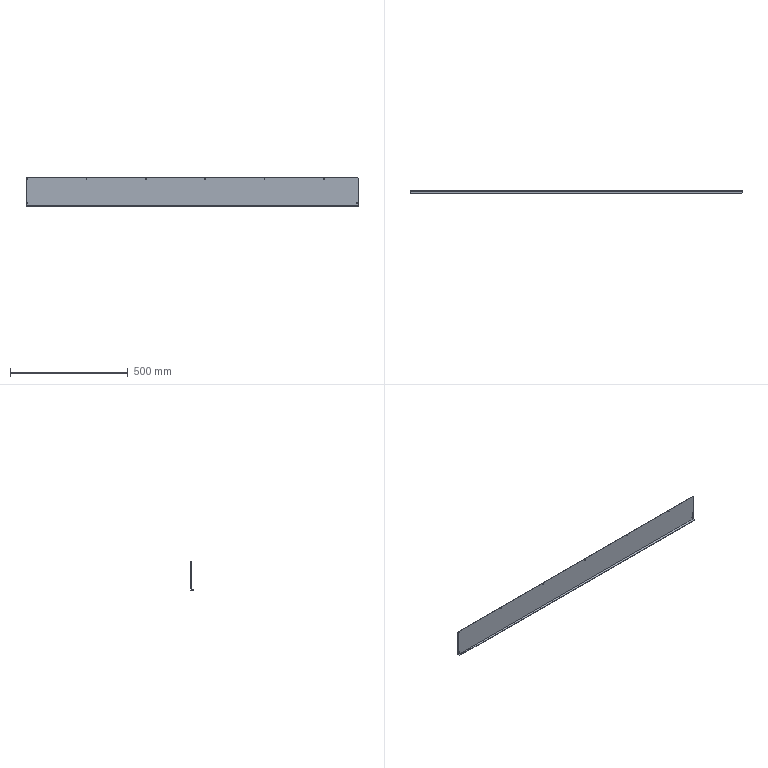Part | NX | 1 solid | 20 faces | box 1410 x 10.5 x 119 mm | volume 359389 mm3 | plane 12 | cylinder 8 | commonest cylinder face diameters 3.4 x8
STEP:
#1=CARTESIAN_POINT('',(-705.,0.,-117.));
#2=VERTEX_POINT('',#1);
#3=CARTESIAN_POINT('',(-705.,-6.5,-117.));
#4=VERTEX_POINT('',#3);
#5=CARTESIAN_POINT('',(-705.,0.,-117.));
#6=DIRECTION('',(0.,-1.,0.));
#7=VECTOR('',#6,1000.);
#8=LINE('',#5,#7);
#9=EDGE_CURVE('',#2,#4,#8,.T.);
#10=ORIENTED_EDGE('',*,*,#9,.T.);
#11=CARTESIAN_POINT('',(-703.,-8.5,-117.));
#12=VERTEX_POINT('',#11);
#13=CARTESIAN_POINT('',(-705.,-6.5,-117.));
#14=DIRECTION('',(-0.7071,0.7071,0.));
#15=VECTOR('',#14,1000.);
#16=LINE('',#13,#15);
#17=EDGE_CURVE('',#4,#12,#16,.F.);
#18=ORIENTED_EDGE('',*,*,#17,.T.);
#19=CARTESIAN_POINT('',(703.,-8.5,-117.));
#20=VERTEX_POINT('',#19);
#21=CARTESIAN_POINT('',(705.,-8.5,-117.));
#22=DIRECTION('',(-1.,0.,0.));
#23=VECTOR('',#22,1000.);
#24=LINE('',#21,#23);
#25=EDGE_CURVE('',#20,#12,#24,.T.);
#26=ORIENTED_EDGE('',*,*,#25,.F.);
#27=CARTESIAN_POINT('',(705.,-6.5,-117.));
#28=VERTEX_POINT('',#27);
#29=CARTESIAN_POINT('',(703.,-8.5,-117.));
#30=DIRECTION('',(0.7071,0.7071,0.));
#31=VECTOR('',#30,1000.);
#32=LINE('',#29,#31);
#33=EDGE_CURVE('',#20,#28,#32,.T.);
#34=ORIENTED_EDGE('',*,*,#33,.T.);
#35=CARTESIAN_POINT('',(705.,0.,-117.));
#36=VERTEX_POINT('',#35);
#37=CARTESIAN_POINT('',(705.,0.,-117.));
#38=DIRECTION('',(0.,-1.,0.));
#39=VECTOR('',#38,1000.);
#40=LINE('',#37,#39);
#41=EDGE_CURVE('',#36,#28,#40,.T.);
#42=ORIENTED_EDGE('',*,*,#41,.F.);
#43=CARTESIAN_POINT('',(705.,0.,-117.));
#44=DIRECTION('',(-1.,0.,0.));
#45=VECTOR('',#44,1000.);
#46=LINE('',#43,#45);
#47=EDGE_CURVE('',#36,#2,#46,.T.);
#48=ORIENTED_EDGE('',*,*,#47,.T.);
#49=EDGE_LOOP('',(#10,#18,#26,#34,#42,#48));
#50=FACE_BOUND('',#49,.T.);
#51=CARTESIAN_POINT('',(705.,0.,-117.));
#52=DIRECTION('',(0.,0.,-1.));
#53=DIRECTION('',(-1.,0.,0.));
#54=AXIS2_PLACEMENT_3D('',#51,#52,#53);
#55=PLANE('',#54);
#56=ADVANCED_FACE('',(#50),#55,.F.);
#57=ORIENTED_EDGE('',*,*,#25,.T.);
#58=CARTESIAN_POINT('',(-703.,-8.5,-119.));
#59=VERTEX_POINT('',#58);
#60=CARTESIAN_POINT('',(-703.,-8.5,-119.));
#61=DIRECTION('',(0.,0.,-1.));
#62=VECTOR('',#61,1000.);
#63=LINE('',#60,#62);
#64=EDGE_CURVE('',#12,#59,#63,.T.);
#65=ORIENTED_EDGE('',*,*,#64,.T.);
#66=CARTESIAN_POINT('',(703.,-8.5,-119.));
#67=VERTEX_POINT('',#66);
#68=CARTESIAN_POINT('',(705.,-8.5,-119.));
#69=DIRECTION('',(-1.,0.,0.));
#70=VECTOR('',#69,1000.);
#71=LINE('',#68,#70);
#72=EDGE_CURVE('',#67,#59,#71,.T.);
#73=ORIENTED_EDGE('',*,*,#72,.F.);
#74=CARTESIAN_POINT('',(703.,-8.5,-117.));
#75=DIRECTION('',(0.,0.,1.));
#76=VECTOR('',#75,1000.);
#77=LINE('',#74,#76);
#78=EDGE_CURVE('',#67,#20,#77,.T.);
#79=ORIENTED_EDGE('',*,*,#78,.T.);
#80=EDGE_LOOP('',(#57,#65,#73,#79));
#81=FACE_BOUND('',#80,.T.);
#82=CARTESIAN_POINT('',(705.,-8.5,-119.));
#83=DIRECTION('',(0.,-1.,0.));
#84=DIRECTION('',(0.,0.,-1.));
#85=AXIS2_PLACEMENT_3D('',#82,#83,#84);
#86=PLANE('',#85);
#87=ADVANCED_FACE('',(#81),#86,.T.);
#88=ORIENTED_EDGE('',*,*,#72,.T.);
#89=CARTESIAN_POINT('',(-705.,-6.5,-119.));
#90=VERTEX_POINT('',#89);
#91=CARTESIAN_POINT('',(-3.25,-708.25,-119.));
#92=DIRECTION('',(0.7071,-0.7071,0.));
#93=VECTOR('',#92,1000.);
#94=LINE('',#91,#93);
#95=EDGE_CURVE('',#59,#90,#94,.F.);
#96=ORIENTED_EDGE('',*,*,#95,.T.);
#97=CARTESIAN_POINT('',(-705.,2.,-119.));
#98=VERTEX_POINT('',#97);
#99=CARTESIAN_POINT('',(-705.,0.,-119.));
#100=DIRECTION('',(0.,1.,0.));
#101=VECTOR('',#100,1000.);
#102=LINE('',#99,#101);
#103=EDGE_CURVE('',#98,#90,#102,.F.);
#104=ORIENTED_EDGE('',*,*,#103,.F.);
#105=CARTESIAN_POINT('',(705.,2.,-119.));
#106=VERTEX_POINT('',#105);
#107=CARTESIAN_POINT('',(705.,2.,-119.));
#108=DIRECTION('',(-1.,0.,0.));
#109=VECTOR('',#108,1000.);
#110=LINE('',#107,#109);
#111=EDGE_CURVE('',#106,#98,#110,.T.);
#112=ORIENTED_EDGE('',*,*,#111,.F.);
#113=CARTESIAN_POINT('',(705.,-6.5,-119.));
#114=VERTEX_POINT('',#113);
#115=CARTESIAN_POINT('',(705.,0.,-119.));
#116=DIRECTION('',(0.,1.,0.));
#117=VECTOR('',#116,1000.);
#118=LINE('',#115,#117);
#119=EDGE_CURVE('',#106,#114,#118,.F.);
#120=ORIENTED_EDGE('',*,*,#119,.T.);
#121=CARTESIAN_POINT('',(708.25,-3.25,-119.));
#122=DIRECTION('',(-0.7071,-0.7071,0.));
#123=VECTOR('',#122,1000.);
#124=LINE('',#121,#123);
#125=EDGE_CURVE('',#114,#67,#124,.T.);
#126=ORIENTED_EDGE('',*,*,#125,.T.);
#127=EDGE_LOOP('',(#88,#96,#104,#112,#120,#126));
#128=FACE_BOUND('',#127,.T.);
#129=CARTESIAN_POINT('',(705.,0.,-119.));
#130=DIRECTION('',(0.,0.,-1.));
#131=DIRECTION('',(-1.,0.,0.));
#132=AXIS2_PLACEMENT_3D('',#129,#130,#131);
#133=PLANE('',#132);
#134=ADVANCED_FACE('',(#128),#133,.T.);
#135=CARTESIAN_POINT('',(-700.,2.,-103.3));
#136=VERTEX_POINT('',#135);
#137=CARTESIAN_POINT('',(-700.,2.,-105.));
#138=DIRECTION('',(0.,1.,0.));
#139=DIRECTION('',(0.,0.,1.));
#140=AXIS2_PLACEMENT_3D('',#137,#138,#139);
#141=CIRCLE('',#140,1.7);
#142=EDGE_CURVE('',#136,#136,#141,.T.);
#143=ORIENTED_EDGE('',*,*,#142,.F.);
#144=EDGE_LOOP('',(#143));
#145=FACE_BOUND('',#144,.T.);
#146=CARTESIAN_POINT('',(700.,2.,-103.3));
#147=VERTEX_POINT('',#146);
#148=CARTESIAN_POINT('',(700.,2.,-105.));
#149=DIRECTION('',(0.,1.,0.));
#150=DIRECTION('',(0.,0.,1.));
#151=AXIS2_PLACEMENT_3D('',#148,#149,#150);
#152=CIRCLE('',#151,1.7);
#153=EDGE_CURVE('',#147,#147,#152,.T.);
#154=ORIENTED_EDGE('',*,*,#153,.F.);
#155=EDGE_LOOP('',(#154));
#156=FACE_BOUND('',#155,.T.);
#157=CARTESIAN_POINT('',(-448.,2.,-3.3));
#158=VERTEX_POINT('',#157);
#159=CARTESIAN_POINT('',(-448.,2.,-5.));
#160=DIRECTION('',(0.,1.,0.));
#161=DIRECTION('',(0.,0.,1.));
#162=AXIS2_PLACEMENT_3D('',#159,#160,#161);
#163=CIRCLE('',#162,1.7);
#164=EDGE_CURVE('',#158,#158,#163,.T.);
#165=ORIENTED_EDGE('',*,*,#164,.F.);
#166=EDGE_LOOP('',(#165));
#167=FACE_BOUND('',#166,.T.);
#168=CARTESIAN_POINT('',(-700.,2.,-3.3));
#169=VERTEX_POINT('',#168);
#170=CARTESIAN_POINT('',(-700.,2.,-5.));
#171=DIRECTION('',(0.,1.,0.));
#172=DIRECTION('',(0.,0.,1.));
#173=AXIS2_PLACEMENT_3D('',#170,#171,#172);
#174=CIRCLE('',#173,1.7);
#175=EDGE_CURVE('',#169,#169,#174,.T.);
#176=ORIENTED_EDGE('',*,*,#175,.F.);
#177=EDGE_LOOP('',(#176));
#178=FACE_BOUND('',#177,.T.);
#179=CARTESIAN_POINT('',(703.,2.,0.));
#180=VERTEX_POINT('',#179);
#181=CARTESIAN_POINT('',(-703.,2.,0.));
#182=VERTEX_POINT('',#181);
#183=CARTESIAN_POINT('',(705.,2.,0.));
#184=DIRECTION('',(-1.,0.,0.));
#185=VECTOR('',#184,1000.);
#186=LINE('',#183,#185);
#187=EDGE_CURVE('',#180,#182,#186,.T.);
#188=ORIENTED_EDGE('',*,*,#187,.F.);
#189=CARTESIAN_POINT('',(705.,2.,-2.));
#190=VERTEX_POINT('',#189);
#191=CARTESIAN_POINT('',(704.,2.,-1.));
#192=DIRECTION('',(0.7071,0.,-0.7071));
#193=VECTOR('',#192,1000.);
#194=LINE('',#191,#193);
#195=EDGE_CURVE('',#180,#190,#194,.T.);
#196=ORIENTED_EDGE('',*,*,#195,.T.);
#197=CARTESIAN_POINT('',(705.,2.,0.));
#198=DIRECTION('',(0.,0.,-1.));
#199=VECTOR('',#198,1000.);
#200=LINE('',#197,#199);
#201=EDGE_CURVE('',#190,#106,#200,.T.);
#202=ORIENTED_EDGE('',*,*,#201,.T.);
#203=ORIENTED_EDGE('',*,*,#111,.T.);
#204=CARTESIAN_POINT('',(-705.,2.,-2.));
#205=VERTEX_POINT('',#204);
#206=CARTESIAN_POINT('',(-705.,2.,0.));
#207=DIRECTION('',(0.,0.,-1.));
#208=VECTOR('',#207,1000.);
#209=LINE('',#206,#208);
#210=EDGE_CURVE('',#205,#98,#209,.T.);
#211=ORIENTED_EDGE('',*,*,#210,.F.);
#212=CARTESIAN_POINT('',(1.,2.,704.));
#213=DIRECTION('',(-0.7071,0.,-0.7071));
#214=VECTOR('',#213,1000.);
#215=LINE('',#212,#214);
#216=EDGE_CURVE('',#205,#182,#215,.F.);
#217=ORIENTED_EDGE('',*,*,#216,.T.);
#218=EDGE_LOOP('',(#188,#196,#202,#203,#211,#217));
#219=FACE_BOUND('',#218,.T.);
#220=CARTESIAN_POINT('',(-196.,2.,-3.3));
#221=VERTEX_POINT('',#220);
#222=CARTESIAN_POINT('',(-196.,2.,-5.));
#223=DIRECTION('',(0.,1.,0.));
#224=DIRECTION('',(0.,0.,1.));
#225=AXIS2_PLACEMENT_3D('',#222,#223,#224);
#226=CIRCLE('',#225,1.7);
#227=EDGE_CURVE('',#221,#221,#226,.T.);
#228=ORIENTED_EDGE('',*,*,#227,.F.);
#229=EDGE_LOOP('',(#228));
#230=FACE_BOUND('',#229,.T.);
#231=CARTESIAN_POINT('',(56.,2.,-3.3));
#232=VERTEX_POINT('',#231);
#233=CARTESIAN_POINT('',(56.,2.,-5.));
#234=DIRECTION('',(0.,1.,0.));
#235=DIRECTION('',(0.,0.,1.));
#236=AXIS2_PLACEMENT_3D('',#233,#234,#235);
#237=CIRCLE('',#236,1.7);
#238=EDGE_CURVE('',#232,#232,#237,.T.);
#239=ORIENTED_EDGE('',*,*,#238,.F.);
#240=EDGE_LOOP('',(#239));
#241=FACE_BOUND('',#240,.T.);
#242=CARTESIAN_POINT('',(308.,2.,-3.3));
#243=VERTEX_POINT('',#242);
#244=CARTESIAN_POINT('',(308.,2.,-5.));
#245=DIRECTION('',(0.,1.,0.));
#246=DIRECTION('',(0.,0.,1.));
#247=AXIS2_PLACEMENT_3D('',#244,#245,#246);
#248=CIRCLE('',#247,1.7);
#249=EDGE_CURVE('',#243,#243,#248,.T.);
#250=ORIENTED_EDGE('',*,*,#249,.F.);
#251=EDGE_LOOP('',(#250));
#252=FACE_BOUND('',#251,.T.);
#253=CARTESIAN_POINT('',(560.,2.,-3.3));
#254=VERTEX_POINT('',#253);
#255=CARTESIAN_POINT('',(560.,2.,-5.));
#256=DIRECTION('',(0.,1.,0.));
#257=DIRECTION('',(0.,0.,1.));
#258=AXIS2_PLACEMENT_3D('',#255,#256,#257);
#259=CIRCLE('',#258,1.7);
#260=EDGE_CURVE('',#254,#254,#259,.T.);
#261=ORIENTED_EDGE('',*,*,#260,.F.);
#262=EDGE_LOOP('',(#261));
#263=FACE_BOUND('',#262,.T.);
#264=CARTESIAN_POINT('',(705.,2.,0.));
#265=DIRECTION('',(0.,1.,0.));
#266=DIRECTION('',(0.,0.,1.));
#267=AXIS2_PLACEMENT_3D('',#264,#265,#266);
#268=PLANE('',#267);
#269=ADVANCED_FACE('',(#145,#156,#167,#178,#219,#230,#241,#252,#263),#268,.T.);
#270=CARTESIAN_POINT('',(703.,0.,0.));
#271=VERTEX_POINT('',#270);
#272=CARTESIAN_POINT('',(-703.,0.,0.));
#273=VERTEX_POINT('',#272);
#274=CARTESIAN_POINT('',(705.,0.,0.));
#275=DIRECTION('',(-1.,0.,0.));
#276=VECTOR('',#275,1000.);
#277=LINE('',#274,#276);
#278=EDGE_CURVE('',#271,#273,#277,.T.);
#279=ORIENTED_EDGE('',*,*,#278,.F.);
#280=CARTESIAN_POINT('',(703.,2.,0.));
#281=DIRECTION('',(0.,1.,0.));
#282=VECTOR('',#281,1000.);
#283=LINE('',#280,#282);
#284=EDGE_CURVE('',#271,#180,#283,.T.);
#285=ORIENTED_EDGE('',*,*,#284,.T.);
#286=ORIENTED_EDGE('',*,*,#187,.T.);
#287=CARTESIAN_POINT('',(-703.,0.,0.));
#288=DIRECTION('',(0.,-1.,0.));
#289=VECTOR('',#288,1000.);
#290=LINE('',#287,#289);
#291=EDGE_CURVE('',#182,#273,#290,.T.);
#292=ORIENTED_EDGE('',*,*,#291,.T.);
#293=EDGE_LOOP('',(#279,#285,#286,#292));
#294=FACE_BOUND('',#293,.T.);
#295=CARTESIAN_POINT('',(705.,0.,0.));
#296=DIRECTION('',(0.,0.,1.));
#297=DIRECTION('',(1.,0.,0.));
#298=AXIS2_PLACEMENT_3D('',#295,#296,#297);
#299=PLANE('',#298);
#300=ADVANCED_FACE('',(#294),#299,.T.);
#301=CARTESIAN_POINT('',(-700.,0.,-103.3));
#302=VERTEX_POINT('',#301);
#303=CARTESIAN_POINT('',(-700.,0.,-105.));
#304=DIRECTION('',(0.,1.,0.));
#305=DIRECTION('',(0.,0.,1.));
#306=AXIS2_PLACEMENT_3D('',#303,#304,#305);
#307=CIRCLE('',#306,1.7);
#308=EDGE_CURVE('',#302,#302,#307,.T.);
#309=ORIENTED_EDGE('',*,*,#308,.T.);
#310=EDGE_LOOP('',(#309));
#311=FACE_BOUND('',#310,.T.);
#312=CARTESIAN_POINT('',(700.,0.,-103.3));
#313=VERTEX_POINT('',#312);
#314=CARTESIAN_POINT('',(700.,0.,-105.));
#315=DIRECTION('',(0.,1.,0.));
#316=DIRECTION('',(0.,0.,1.));
#317=AXIS2_PLACEMENT_3D('',#314,#315,#316);
#318=CIRCLE('',#317,1.7);
#319=EDGE_CURVE('',#313,#313,#318,.T.);
#320=ORIENTED_EDGE('',*,*,#319,.T.);
#321=EDGE_LOOP('',(#320));
#322=FACE_BOUND('',#321,.T.);
#323=CARTESIAN_POINT('',(-448.,0.,-3.3));
#324=VERTEX_POINT('',#323);
#325=CARTESIAN_POINT('',(-448.,0.,-5.));
#326=DIRECTION('',(0.,1.,0.));
#327=DIRECTION('',(0.,0.,1.));
#328=AXIS2_PLACEMENT_3D('',#325,#326,#327);
#329=CIRCLE('',#328,1.7);
#330=EDGE_CURVE('',#324,#324,#329,.T.);
#331=ORIENTED_EDGE('',*,*,#330,.T.);
#332=EDGE_LOOP('',(#331));
#333=FACE_BOUND('',#332,.T.);
#334=CARTESIAN_POINT('',(-700.,0.,-3.3));
#335=VERTEX_POINT('',#334);
#336=CARTESIAN_POINT('',(-700.,0.,-5.));
#337=DIRECTION('',(0.,1.,0.));
#338=DIRECTION('',(0.,0.,1.));
#339=AXIS2_PLACEMENT_3D('',#336,#337,#338);
#340=CIRCLE('',#339,1.7);
#341=EDGE_CURVE('',#335,#335,#340,.T.);
#342=ORIENTED_EDGE('',*,*,#341,.T.);
#343=EDGE_LOOP('',(#342));
#344=FACE_BOUND('',#343,.T.);
#345=CARTESIAN_POINT('',(705.,0.,-2.));
#346=VERTEX_POINT('',#345);
#347=CARTESIAN_POINT('',(705.,0.,0.));
#348=DIRECTION('',(0.,0.,-1.));
#349=VECTOR('',#348,1000.);
#350=LINE('',#347,#349);
#351=EDGE_CURVE('',#346,#36,#350,.T.);
#352=ORIENTED_EDGE('',*,*,#351,.F.);
#353=CARTESIAN_POINT('',(703.,0.,0.));
#354=DIRECTION('',(-0.7071,0.,0.7071));
#355=VECTOR('',#354,1000.);
#356=LINE('',#353,#355);
#357=EDGE_CURVE('',#346,#271,#356,.T.);
#358=ORIENTED_EDGE('',*,*,#357,.T.);
#359=ORIENTED_EDGE('',*,*,#278,.T.);
#360=CARTESIAN_POINT('',(-705.,0.,-2.));
#361=VERTEX_POINT('',#360);
#362=CARTESIAN_POINT('',(-705.,0.,-2.));
#363=DIRECTION('',(0.7071,0.,0.7071));
#364=VECTOR('',#363,1000.);
#365=LINE('',#362,#364);
#366=EDGE_CURVE('',#273,#361,#365,.F.);
#367=ORIENTED_EDGE('',*,*,#366,.T.);
#368=CARTESIAN_POINT('',(-705.,0.,0.));
#369=DIRECTION('',(0.,0.,-1.));
#370=VECTOR('',#369,1000.);
#371=LINE('',#368,#370);
#372=EDGE_CURVE('',#361,#2,#371,.T.);
#373=ORIENTED_EDGE('',*,*,#372,.T.);
#374=ORIENTED_EDGE('',*,*,#47,.F.);
#375=EDGE_LOOP('',(#352,#358,#359,#367,#373,#374));
#376=FACE_BOUND('',#375,.T.);
#377=CARTESIAN_POINT('',(-196.,0.,-3.3));
#378=VERTEX_POINT('',#377);
#379=CARTESIAN_POINT('',(-196.,0.,-5.));
#380=DIRECTION('',(0.,1.,0.));
#381=DIRECTION('',(0.,0.,1.));
#382=AXIS2_PLACEMENT_3D('',#379,#380,#381);
#383=CIRCLE('',#382,1.7);
#384=EDGE_CURVE('',#378,#378,#383,.T.);
#385=ORIENTED_EDGE('',*,*,#384,.T.);
#386=EDGE_LOOP('',(#385));
#387=FACE_BOUND('',#386,.T.);
#388=CARTESIAN_POINT('',(56.,0.,-3.3));
#389=VERTEX_POINT('',#388);
#390=CARTESIAN_POINT('',(56.,0.,-5.));
#391=DIRECTION('',(0.,1.,0.));
#392=DIRECTION('',(0.,0.,1.));
#393=AXIS2_PLACEMENT_3D('',#390,#391,#392);
#394=CIRCLE('',#393,1.7);
#395=EDGE_CURVE('',#389,#389,#394,.T.);
#396=ORIENTED_EDGE('',*,*,#395,.T.);
#397=EDGE_LOOP('',(#396));
#398=FACE_BOUND('',#397,.T.);
#399=CARTESIAN_POINT('',(308.,0.,-3.3));
#400=VERTEX_POINT('',#399);
#401=CARTESIAN_POINT('',(308.,0.,-5.));
#402=DIRECTION('',(0.,1.,0.));
#403=DIRECTION('',(0.,0.,1.));
#404=AXIS2_PLACEMENT_3D('',#401,#402,#403);
#405=CIRCLE('',#404,1.7);
#406=EDGE_CURVE('',#400,#400,#405,.T.);
#407=ORIENTED_EDGE('',*,*,#406,.T.);
#408=EDGE_LOOP('',(#407));
#409=FACE_BOUND('',#408,.T.);
#410=CARTESIAN_POINT('',(560.,0.,-3.3));
#411=VERTEX_POINT('',#410);
#412=CARTESIAN_POINT('',(560.,0.,-5.));
#413=DIRECTION('',(0.,1.,0.));
#414=DIRECTION('',(0.,0.,1.));
#415=AXIS2_PLACEMENT_3D('',#412,#413,#414);
#416=CIRCLE('',#415,1.7);
#417=EDGE_CURVE('',#411,#411,#416,.T.);
#418=ORIENTED_EDGE('',*,*,#417,.T.);
#419=EDGE_LOOP('',(#418));
#420=FACE_BOUND('',#419,.T.);
#421=CARTESIAN_POINT('',(705.,0.,0.));
#422=DIRECTION('',(0.,1.,0.));
#423=DIRECTION('',(0.,0.,1.));
#424=AXIS2_PLACEMENT_3D('',#421,#422,#423);
#425=PLANE('',#424);
#426=ADVANCED_FACE('',(#311,#322,#333,#344,#376,#387,#398,#409,#420),#425,.F.);
#427=ORIENTED_EDGE('',*,*,#201,.F.);
#428=CARTESIAN_POINT('',(705.,0.,-2.));
#429=DIRECTION('',(0.,-1.,0.));
#430=VECTOR('',#429,1000.);
#431=LINE('',#428,#430);
#432=EDGE_CURVE('',#190,#346,#431,.T.);
#433=ORIENTED_EDGE('',*,*,#432,.T.);
#434=ORIENTED_EDGE('',*,*,#351,.T.);
#435=ORIENTED_EDGE('',*,*,#41,.T.);
#436=CARTESIAN_POINT('',(705.,-6.5,-119.));
#437=DIRECTION('',(0.,0.,-1.));
#438=VECTOR('',#437,1000.);
#439=LINE('',#436,#438);
#440=EDGE_CURVE('',#28,#114,#439,.T.);
#441=ORIENTED_EDGE('',*,*,#440,.T.);
#442=ORIENTED_EDGE('',*,*,#119,.F.);
#443=EDGE_LOOP('',(#427,#433,#434,#435,#441,#442));
#444=FACE_BOUND('',#443,.T.);
#445=CARTESIAN_POINT('',(705.,0.,0.));
#446=DIRECTION('',(-1.,0.,0.));
#447=DIRECTION('',(0.,0.,1.));
#448=AXIS2_PLACEMENT_3D('',#445,#446,#447);
#449=PLANE('',#448);
#450=ADVANCED_FACE('',(#444),#449,.F.);
#451=ORIENTED_EDGE('',*,*,#372,.F.);
#452=CARTESIAN_POINT('',(-705.,0.,-2.));
#453=DIRECTION('',(0.,1.,0.));
#454=VECTOR('',#453,1000.);
#455=LINE('',#452,#454);
#456=EDGE_CURVE('',#361,#205,#455,.T.);
#457=ORIENTED_EDGE('',*,*,#456,.T.);
#458=ORIENTED_EDGE('',*,*,#210,.T.);
#459=ORIENTED_EDGE('',*,*,#103,.T.);
#460=CARTESIAN_POINT('',(-705.,-6.5,0.));
#461=DIRECTION('',(0.,0.,1.));
#462=VECTOR('',#461,1000.);
#463=LINE('',#460,#462);
#464=EDGE_CURVE('',#90,#4,#463,.T.);
#465=ORIENTED_EDGE('',*,*,#464,.T.);
#466=ORIENTED_EDGE('',*,*,#9,.F.);
#467=EDGE_LOOP('',(#451,#457,#458,#459,#465,#466));
#468=FACE_BOUND('',#467,.T.);
#469=CARTESIAN_POINT('',(-705.,0.,0.));
#470=DIRECTION('',(-1.,0.,0.));
#471=DIRECTION('',(0.,0.,1.));
#472=AXIS2_PLACEMENT_3D('',#469,#470,#471);
#473=PLANE('',#472);
#474=ADVANCED_FACE('',(#468),#473,.T.);
#475=ORIENTED_EDGE('',*,*,#357,.F.);
#476=ORIENTED_EDGE('',*,*,#432,.F.);
#477=ORIENTED_EDGE('',*,*,#195,.F.);
#478=ORIENTED_EDGE('',*,*,#284,.F.);
#479=EDGE_LOOP('',(#475,#476,#477,#478));
#480=FACE_BOUND('',#479,.T.);
#481=CARTESIAN_POINT('',(703.,0.,0.));
#482=DIRECTION('',(0.7071,0.,0.7071));
#483=DIRECTION('',(0.,-1.,0.));
#484=AXIS2_PLACEMENT_3D('',#481,#482,#483);
#485=PLANE('',#484);
#486=ADVANCED_FACE('',(#480),#485,.T.);
#487=ORIENTED_EDGE('',*,*,#366,.F.);
#488=ORIENTED_EDGE('',*,*,#291,.F.);
#489=ORIENTED_EDGE('',*,*,#216,.F.);
#490=ORIENTED_EDGE('',*,*,#456,.F.);
#491=EDGE_LOOP('',(#487,#488,#489,#490));
#492=FACE_BOUND('',#491,.T.);
#493=CARTESIAN_POINT('',(-705.,0.,-2.));
#494=DIRECTION('',(0.7071,0.,-0.7071));
#495=DIRECTION('',(0.,1.,0.));
#496=AXIS2_PLACEMENT_3D('',#493,#494,#495);
#497=PLANE('',#496);
#498=ADVANCED_FACE('',(#492),#497,.F.);
#499=ORIENTED_EDGE('',*,*,#95,.F.);
#500=ORIENTED_EDGE('',*,*,#64,.F.);
#501=ORIENTED_EDGE('',*,*,#17,.F.);
#502=ORIENTED_EDGE('',*,*,#464,.F.);
#503=EDGE_LOOP('',(#499,#500,#501,#502));
#504=FACE_BOUND('',#503,.T.);
#505=CARTESIAN_POINT('',(-705.,-6.5,0.));
#506=DIRECTION('',(0.7071,0.7071,0.));
#507=DIRECTION('',(0.,0.,1.));
#508=AXIS2_PLACEMENT_3D('',#505,#506,#507);
#509=PLANE('',#508);
#510=ADVANCED_FACE('',(#504),#509,.F.);
#511=ORIENTED_EDGE('',*,*,#125,.F.);
#512=ORIENTED_EDGE('',*,*,#440,.F.);
#513=ORIENTED_EDGE('',*,*,#33,.F.);
#514=ORIENTED_EDGE('',*,*,#78,.F.);
#515=EDGE_LOOP('',(#511,#512,#513,#514));
#516=FACE_BOUND('',#515,.T.);
#517=CARTESIAN_POINT('',(703.,-8.5,-119.));
#518=DIRECTION('',(0.7071,-0.7071,0.));
#519=DIRECTION('',(0.,0.,-1.));
#520=AXIS2_PLACEMENT_3D('',#517,#518,#519);
#521=PLANE('',#520);
#522=ADVANCED_FACE('',(#516),#521,.T.);
#523=ORIENTED_EDGE('',*,*,#175,.T.);
#524=EDGE_LOOP('',(#523));
#525=FACE_BOUND('',#524,.T.);
#526=ORIENTED_EDGE('',*,*,#341,.F.);
#527=EDGE_LOOP('',(#526));
#528=FACE_BOUND('',#527,.T.);
#529=CARTESIAN_POINT('',(-700.,2.,-5.));
#530=DIRECTION('',(0.,1.,0.));
#531=DIRECTION('',(0.,0.,1.));
#532=AXIS2_PLACEMENT_3D('',#529,#530,#531);
#533=CYLINDRICAL_SURFACE('',#532,1.7);
#534=ADVANCED_FACE('',(#525,#528),#533,.F.);
#535=ORIENTED_EDGE('',*,*,#164,.T.);
#536=EDGE_LOOP('',(#535));
#537=FACE_BOUND('',#536,.T.);
#538=ORIENTED_EDGE('',*,*,#330,.F.);
#539=EDGE_LOOP('',(#538));
#540=FACE_BOUND('',#539,.T.);
#541=CARTESIAN_POINT('',(-448.,2.,-5.));
#542=DIRECTION('',(0.,1.,0.));
#543=DIRECTION('',(0.,0.,1.));
#544=AXIS2_PLACEMENT_3D('',#541,#542,#543);
#545=CYLINDRICAL_SURFACE('',#544,1.7);
#546=ADVANCED_FACE('',(#537,#540),#545,.F.);
#547=ORIENTED_EDGE('',*,*,#227,.T.);
#548=EDGE_LOOP('',(#547));
#549=FACE_BOUND('',#548,.T.);
#550=ORIENTED_EDGE('',*,*,#384,.F.);
#551=EDGE_LOOP('',(#550));
#552=FACE_BOUND('',#551,.T.);
#553=CARTESIAN_POINT('',(-196.,2.,-5.));
#554=DIRECTION('',(0.,1.,0.));
#555=DIRECTION('',(0.,0.,1.));
#556=AXIS2_PLACEMENT_3D('',#553,#554,#555);
#557=CYLINDRICAL_SURFACE('',#556,1.7);
#558=ADVANCED_FACE('',(#549,#552),#557,.F.);
#559=ORIENTED_EDGE('',*,*,#238,.T.);
#560=EDGE_LOOP('',(#559));
#561=FACE_BOUND('',#560,.T.);
#562=ORIENTED_EDGE('',*,*,#395,.F.);
#563=EDGE_LOOP('',(#562));
#564=FACE_BOUND('',#563,.T.);
#565=CARTESIAN_POINT('',(56.,2.,-5.));
#566=DIRECTION('',(0.,1.,0.));
#567=DIRECTION('',(0.,0.,1.));
#568=AXIS2_PLACEMENT_3D('',#565,#566,#567);
#569=CYLINDRICAL_SURFACE('',#568,1.7);
#570=ADVANCED_FACE('',(#561,#564),#569,.F.);
#571=ORIENTED_EDGE('',*,*,#249,.T.);
#572=EDGE_LOOP('',(#571));
#573=FACE_BOUND('',#572,.T.);
#574=ORIENTED_EDGE('',*,*,#406,.F.);
#575=EDGE_LOOP('',(#574));
#576=FACE_BOUND('',#575,.T.);
#577=CARTESIAN_POINT('',(308.,2.,-5.));
#578=DIRECTION('',(0.,1.,0.));
#579=DIRECTION('',(0.,0.,1.));
#580=AXIS2_PLACEMENT_3D('',#577,#578,#579);
#581=CYLINDRICAL_SURFACE('',#580,1.7);
#582=ADVANCED_FACE('',(#573,#576),#581,.F.);
#583=ORIENTED_EDGE('',*,*,#260,.T.);
#584=EDGE_LOOP('',(#583));
#585=FACE_BOUND('',#584,.T.);
#586=ORIENTED_EDGE('',*,*,#417,.F.);
#587=EDGE_LOOP('',(#586));
#588=FACE_BOUND('',#587,.T.);
#589=CARTESIAN_POINT('',(560.,2.,-5.));
#590=DIRECTION('',(0.,1.,0.));
#591=DIRECTION('',(0.,0.,1.));
#592=AXIS2_PLACEMENT_3D('',#589,#590,#591);
#593=CYLINDRICAL_SURFACE('',#592,1.7);
#594=ADVANCED_FACE('',(#585,#588),#593,.F.);
#595=ORIENTED_EDGE('',*,*,#153,.T.);
#596=EDGE_LOOP('',(#595));
#597=FACE_BOUND('',#596,.T.);
#598=ORIENTED_EDGE('',*,*,#319,.F.);
#599=EDGE_LOOP('',(#598));
#600=FACE_BOUND('',#599,.T.);
#601=CARTESIAN_POINT('',(700.,2.,-105.));
#602=DIRECTION('',(0.,1.,0.));
#603=DIRECTION('',(0.,0.,1.));
#604=AXIS2_PLACEMENT_3D('',#601,#602,#603);
#605=CYLINDRICAL_SURFACE('',#604,1.7);
#606=ADVANCED_FACE('',(#597,#600),#605,.F.);
#607=ORIENTED_EDGE('',*,*,#142,.T.);
#608=EDGE_LOOP('',(#607));
#609=FACE_BOUND('',#608,.T.);
#610=ORIENTED_EDGE('',*,*,#308,.F.);
#611=EDGE_LOOP('',(#610));
#612=FACE_BOUND('',#611,.T.);
#613=CARTESIAN_POINT('',(-700.,2.,-105.));
#614=DIRECTION('',(0.,1.,0.));
#615=DIRECTION('',(0.,0.,1.));
#616=AXIS2_PLACEMENT_3D('',#613,#614,#615);
#617=CYLINDRICAL_SURFACE('',#616,1.7);
#618=ADVANCED_FACE('',(#609,#612),#617,.F.);
#619=CLOSED_SHELL('',(#56,#87,#134,#269,#300,#426,#450,#474,#486,#498,#510,#522,#534,#546,#558,#570,#582,#594,#606,#618));
#620=MANIFOLD_SOLID_BREP('',#619);
#621=(LENGTH_UNIT()NAMED_UNIT(*)SI_UNIT(.MILLI.,.METRE.));
#622=UNCERTAINTY_MEASURE_WITH_UNIT(LENGTH_MEASURE(0.00001),#621,'','');
#623=(NAMED_UNIT(*)PLANE_ANGLE_UNIT()SI_UNIT($,.RADIAN.));
#624=(NAMED_UNIT(*)SI_UNIT($,.STERADIAN.)SOLID_ANGLE_UNIT());
#625=(GEOMETRIC_REPRESENTATION_CONTEXT(3)GLOBAL_UNCERTAINTY_ASSIGNED_CONTEXT((#622))GLOBAL_UNIT_ASSIGNED_CONTEXT((#621,#623,#624))REPRESENTATION_CONTEXT('',''));
#626=ADVANCED_BREP_SHAPE_REPRESENTATION('',(#620),#625);